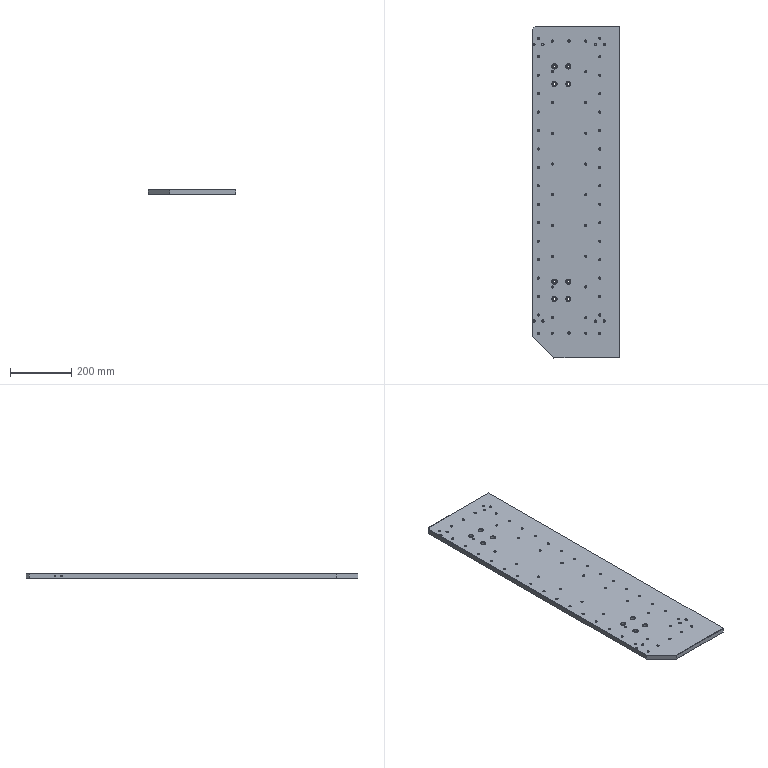Part | SolidWorks | features BaseBody 1 | 1 solid | 494 faces | box 285 x 1080 x 16 mm | volume 4846007 mm3 | cone 300 | cylinder 168 | plane 26 | commonest cylinder face diameters 5 x116 6 x20 8.5 x16 15 x16